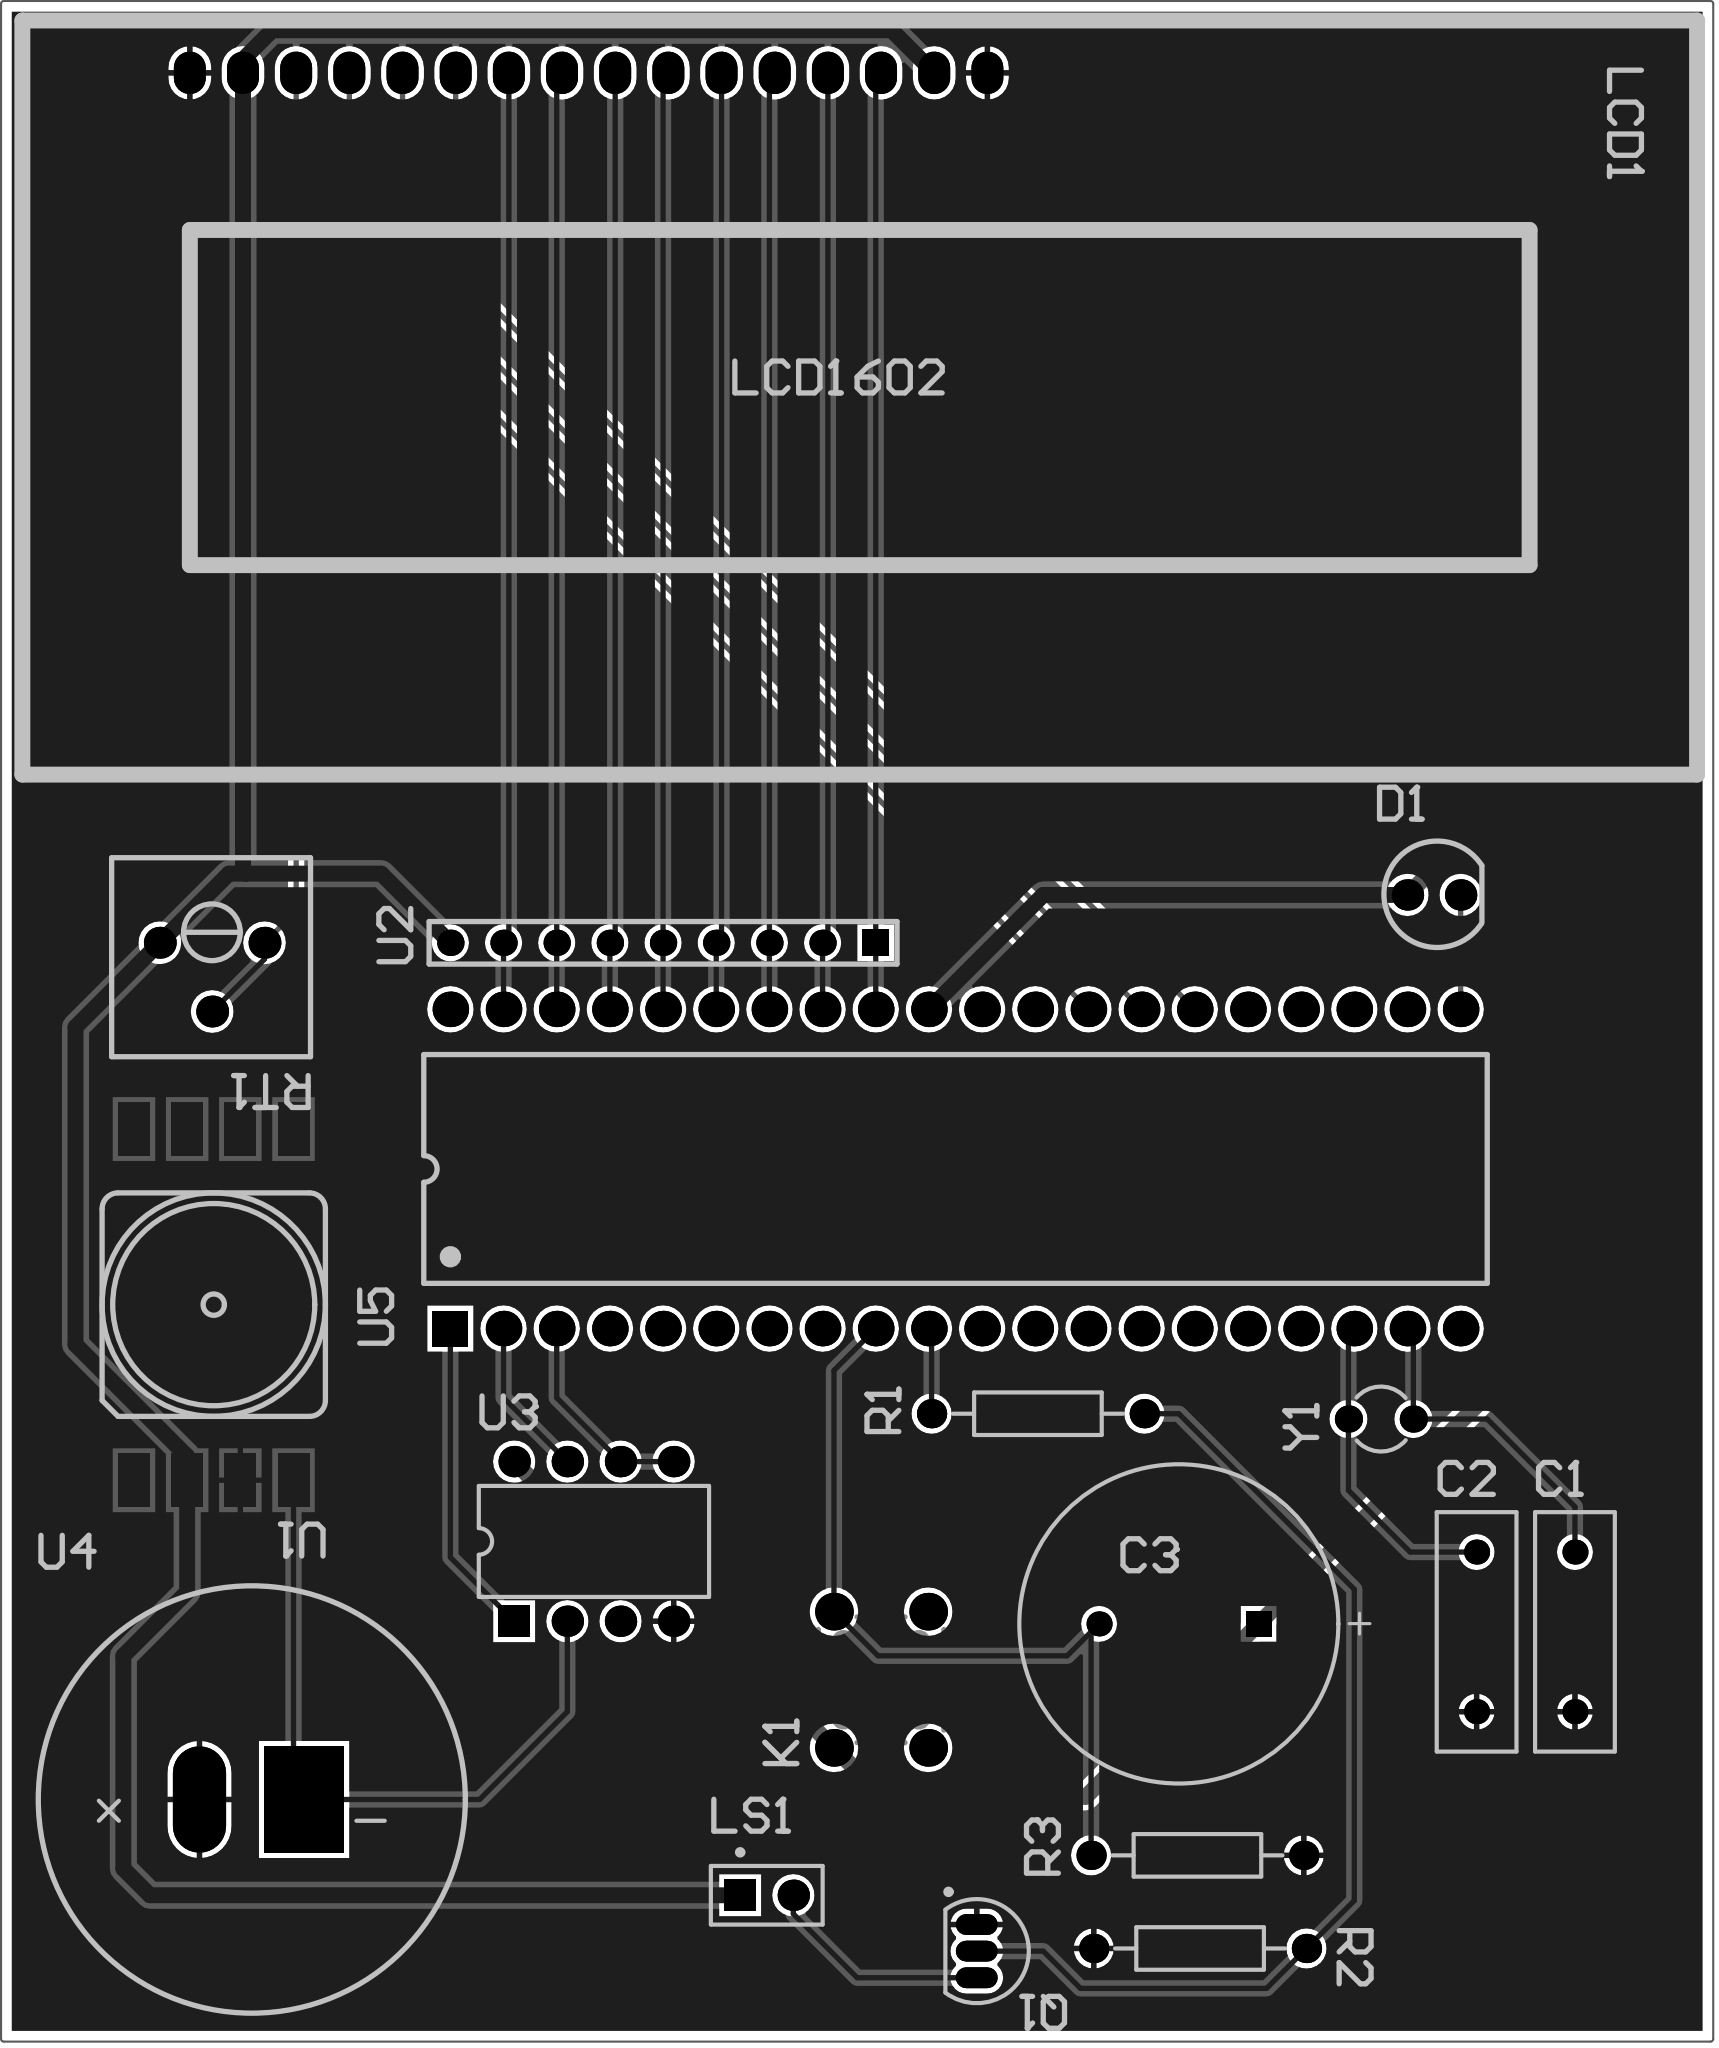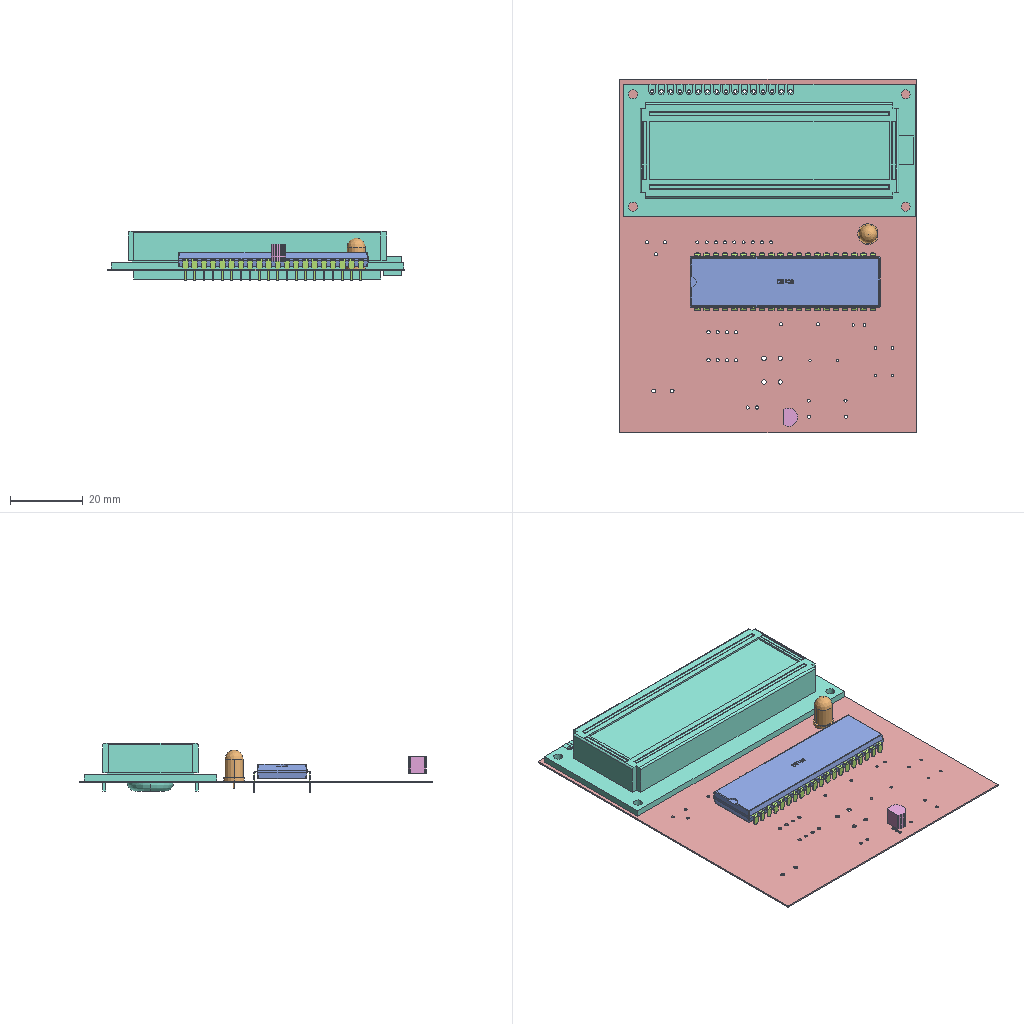Circuit board layout | Altium Designer | box 81.8 x 97.4 x 13.7 mm
Layer stack:
# Altium Designer layer stack of  (unit mm; dielectric type: 0 none, 1 core, 2 prepreg, 3 surface material)
index,name,kind,layer,copper_thickness_mm,dielectric_type,dielectric_thickness_mm,dielectric_material,dielectric_constant
0,Top Paste,other,,,,,,
1,Top Overlay,other,,,,,,
2,Top Solder,dielectric,,,3,0.0102,Solder Resist,3.5
3,Top Layer,copper,Top Layer,0.0356,,,,
4,Dielectric 1,dielectric,,,0,0.32,FR-4,4.8
5,Bottom Layer,copper,Bottom Layer,0.0356,,,,
6,Bottom Solder,dielectric,,,3,0.0102,Solder Resist,3.5
7,Bottom Overlay,other,,,,,,
8,Bottom Paste,other,,,,,,
# drill layer pairs: low layer,high layer
drill_pair,Top Layer,Bottom Layer
Part placement:
Designator,Comment,Layer,Footprint,Center-X(mm),Center-Y(mm),Rotation
Y1,XTAL,TopLayer,R38,120.777,59.436,90
U5,AT89C52,TopLayer,DIP40,100.457,71.374,90
U4,Volts,TopLayer,CAPACITANCE_1_FARAD_5,5_VOLT,66.842,41.275,0
U3,ADC0832,TopLayer,P008,83.185,53.594,0
U2,排阻,TopLayer,paizu,86.487,82.169,180
U1,MPXA6115A6U,TopLayer,482,65.024,64.897,270
RT1,10K,TopLayer,电位器,64.948,80.531,180
R3,10K,TopLayer,AXIAL-0.4,112.014,38.608,180
R2,10K,TopLayer,AXIAL-0.4,112.141,34.163,360
R1,1K,TopLayer,AXIAL-0.4,104.394,59.69,180
Q1,2N3904,TopLayer,TO-92A,101.473,34.036,180
LS1,Bell,TopLayer,PIN2,91.44,36.703,360
LCD1,LCD1602,TopLayer,LCD1602,82.931,123.698,360
K1,HH+,TopLayer,四脚轻触开关,96.901,46.99,90
D1,LED,TopLayer,LED5-BLUE,123.317,84.455,0
C3,10UF,TopLayer,RB7.6-15,111.125,49.657,0
C2,22U,TopLayer,RAD-0.3,125.349,49.276,90
C1,22U,TopLayer,RAD-0.3,130.048,49.276,90
Pad and via stacks:
# Altium Designer via and pad stacks of  (unit mm). Each distinct definition once, with the count of objects using it.
# via: kind,start_layer,end_layer,hole_mm,diameter_mm,mode(0 simple;1 top-mid-bottom;2 full stack),diameter_per_layer,count,example_net
# pad: kind,layer,hole_mm,hole_type(0 round;1 square;2 slot),plating,top_size,top_shape(1 round;2 rect;3 octagon;9 rounded rect),mid_size,bottom_size,mode,footprint,size_per_layer,count,example
pad,Multi-Layer,0.9,0,plated,1.524x2.032,1,1.524x2.032,1.524x2.032,0,LCD1602,,16,LCD1.1
pad,Multi-Layer,0.9,0,plated,1.524x1.524,1,1.524x1.524,1.524x1.524,0,\u00B5\u00E7\u00CE\u00BB\u00C6\u00F7,,3,RT1.3
pad,Multi-Layer,0.84,0,plated,1.26x1.26,2,1.26x1.26,1.26x1.26,0,paizu,,1,U2.1
pad,Multi-Layer,0.84,0,plated,1.26x1.26,1,1.26x1.26,1.26x1.26,0,paizu,,8,U2.2
pad,Multi-Layer,0.9,0,plated,1.5x1.5,2,1.5x1.5,1.5x1.5,0,P008,,1,U3.1
pad,Multi-Layer,0.9,0,plated,1.5x1.5,1,1.5x1.5,1.5x1.5,0,P008,,7,U3.2
pad,Multi-Layer,1.1,0,plated,3.81x5.08,2,3.81x5.08,3.81x5.08,0,CAPACITANCE 1 FARAD 5,5 VOLT,,1,U4.1
pad,Multi-Layer,1.1,0,plated,2.54x5.08,1,2.54x5.08,2.54x5.08,0,CAPACITANCE 1 FARAD 5,5 VOLT,,1,U4.2
pad,Multi-Layer,0.8,0,plated,1.7x1.7,1,1.7x1.7,1.7x1.7,0,DIP40,,39,U5.21
pad,Multi-Layer,0.8,0,plated,1.7x1.7,2,1.7x1.7,1.7x1.7,0,DIP40,,1,U5.1
pad,Multi-Layer,0.7,0,plated,1.2x1.2,1,1.2x1.2,1.2x1.2,0,RAD-0.3,,4,C1.2
pad,Multi-Layer,0.7,0,plated,1.3x1.3,1,1.3x1.3,1.3x1.3,0,R38,,2,Y1.1
pad,Multi-Layer,0.9,0,plated,1.5x1.5,2,1.5x1.5,1.5x1.5,0,PIN2,,1,LS1.1
pad,Multi-Layer,0.9,0,plated,1.5x1.5,1,1.5x1.5,1.5x1.5,0,PIN2,,1,LS1.2
pad,Multi-Layer,0.7,0,plated,1.2x1.2,2,1.2x1.2,1.2x1.2,0,RB7.6-15,,1,C3.1
pad,Multi-Layer,0.7,0,plated,1.2x1.2,1,1.2x1.2,1.2x1.2,0,RB7.6-15,,1,C3.2
pad,Multi-Layer,0.85,0,plated,1.4x1.4,1,1.4x1.4,1.4x1.4,0,AXIAL-0.4,,6,R1.1
pad,Multi-Layer,0.9,0,plated,2x1,1,2x1,2x1,0,TO-92A,,3,Q1.3
pad,Multi-Layer,1.2,0,plated,1.8x1.8,1,1.8x1.8,1.8x1.8,0,\u00CB\u00C4\u00BD\u00C5\u00C7\u00E1\u00B4\u00A5\u00BF\u00AA\u00B9\u00D8,,4,K1.4
pad,Multi-Layer,0.762,0,plated,1.5x1.5,1,1.5x1.5,1.5x1.5,0,LED5-BLUE,,2,D1.K
pad,Top Layer,0,0,plated,2.54x1.524,2,2.54x1.524,2.54x1.524,0,482,,8,U1.6
Copper pours:
name,layer,net,type(0 solid;1 hatched;2 none)
G,Bottom Layer,GND,0
G,Top Layer,GND,0
Design rules, without the lines most boards share:
# Altium Designer design rules of  (exported by Altium Designer, unit mm)
# columns: name | kind | enabled | priority | scope1 | scope2 | descriptor | typed fields (field=value)
SilkToSilkClearance | 55 | enabled | 1 | All | All | Silk to Silk (Clearance=0mil) (All),(All) |
SilkToSolderMaskClearance | 54 | enabled | 1 | IsPad | All | Silk To Solder Mask (Clearance=0mil) (IsPad),(All) |
MinimumSolderMaskSliver | 53 | enabled | 1 | All | All | Minimum Solder Mask Sliver (Gap=0mil) (All),(All) |
HoleToHoleClearance | 52 | enabled | 1 | All | All | Hole To Hole Clearance (Gap=10mil) (All),(All) | gap=0.254
DiffPairsRouting | 51 | enabled | 1 | All | All | Differential Pairs Uncoupled Length using the Gap Constraints (Min=10mil) (Max=10mil) (Prefered=10mil)  and Width Constraints (Min=15mil) (Max=15mil) (Prefered=15mil) (All) |
SolderMaskExpansion | 13 | enabled | 1 | All | All | Solder Mask Expansion (Expansion =4mil) (All) | expansion=0.1016
PasteMaskExpansion | 14 | enabled | 1 | All | All | Paste Mask Expansion (Expansion =0mil) (All) | expansion=0
RoutingVias | 11 | enabled | 1 | All | All | Routing Via (MinHoleWidth=28mil) (MaxHoleWidth=28mil) (PreferredHoleWidth=28mil) (MinWidth=50mil) (MaxWidth=50mil) (PreferedWidth=50mil) (All) | via_min_hole=0.7112 via_max_hole=0.7112 via_preferred_diameter=1.27 via_preferred_hole=0.7112
Width | 2 | enabled | 1 | All | All | Width Constraint (Min=10mil) (Max=30mil) (Preferred=10mil) (All) |
PolygonConnect | 20 | enabled | 1 | All | All | Polygon Connect Rule(Relief Connect )(Conductor Width=10mil) (Relief Angle=90 Angle) (Entries=4) (Air Gap Width=10mil) (All),(All) | connect_style(0=relief,1=direct,2=none)=0 relief_conductor_width=0.254 relief_entries=4
PlaneConnect | 6 | enabled | 1 | All | All | Power Plane Connect Rule(Relief Connect )(Expansion=20mil) (Conductor Width=10mil) (Air Gap=10mil) (Entries=4) (All) | relief_conductor_width=0.254 relief_entries=4 relief_expansion=0.508
Clearance | 0 | enabled | 1 | All | All | Clearance Constraint (Gap=10mil) (All),(All) | gap=0.254
Classes set for this board:
# Altium Designer classes of  (member kind: 0 net, 1 component, 2 from-to, 3 pad, 4 layer, 5 differential pair, 6 design channel, 7 polygon, 8 structure, 9 xSignal)
# columns: class name | member kind | superclass | members
Sheet1 | 1 | no | C1; C2; C3; D1; K1; LCD1; LS1; Q1; R1; R2; R3; RT1; U1; U2; U3; U4; U5; Y1;